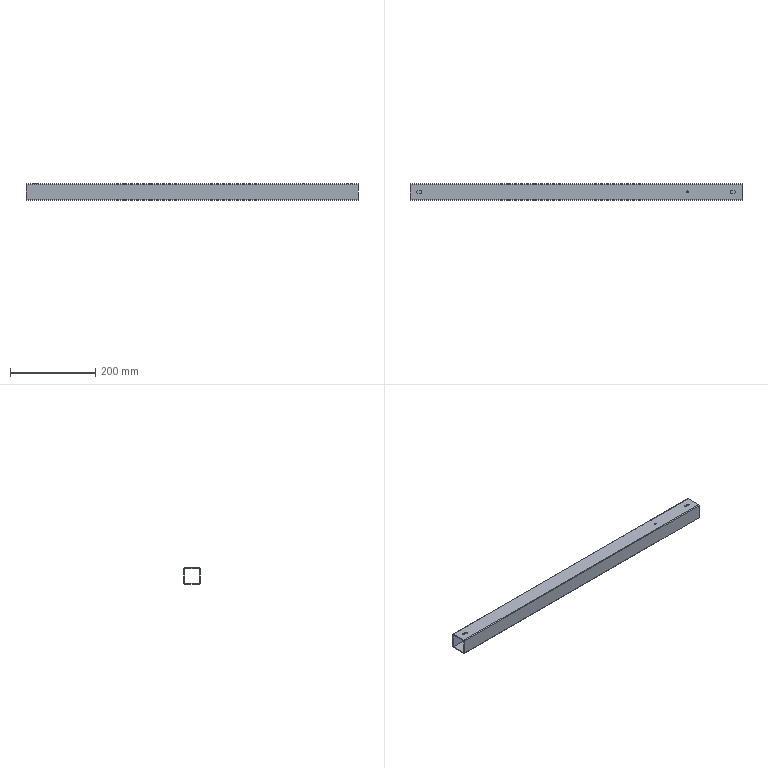Part | NX | features BREP 1 | 1 solid | 26 faces | box 780.034 x 38.1 x 38.1 mm | volume 210452 mm3 | plane 14 | cylinder 12 | commonest cylinder face diameters 5.715 x6 3.175 x4 4.699 x2
STEP:
#1=CARTESIAN_POINT('',(-390.017,19.05,-17.462));
#2=VERTEX_POINT('',#1);
#3=CARTESIAN_POINT('',(-390.017,19.05,17.462));
#4=VERTEX_POINT('',#3);
#5=CARTESIAN_POINT('',(-390.017,19.05,-17.462));
#6=DIRECTION('',(0.,0.,1.));
#7=VECTOR('',#6,1000.);
#8=LINE('',#5,#7);
#9=EDGE_CURVE('',#2,#4,#8,.T.);
#10=ORIENTED_EDGE('',*,*,#9,.F.);
#11=CARTESIAN_POINT('',(-390.017,17.462,-19.05));
#12=VERTEX_POINT('',#11);
#13=CARTESIAN_POINT('',(-390.017,17.462,-17.462));
#14=DIRECTION('',(-1.,0.,0.));
#15=DIRECTION('',(0.,1.,0.));
#16=AXIS2_PLACEMENT_3D('',#13,#14,#15);
#17=CIRCLE('',#16,1.587);
#18=EDGE_CURVE('',#2,#12,#17,.T.);
#19=ORIENTED_EDGE('',*,*,#18,.T.);
#20=CARTESIAN_POINT('',(-390.017,-17.462,-19.05));
#21=VERTEX_POINT('',#20);
#22=CARTESIAN_POINT('',(-390.017,-17.462,-19.05));
#23=DIRECTION('',(0.,1.,0.));
#24=VECTOR('',#23,1000.);
#25=LINE('',#22,#24);
#26=EDGE_CURVE('',#21,#12,#25,.T.);
#27=ORIENTED_EDGE('',*,*,#26,.F.);
#28=CARTESIAN_POINT('',(-390.017,-19.05,-17.462));
#29=VERTEX_POINT('',#28);
#30=CARTESIAN_POINT('',(-390.017,-17.462,-17.462));
#31=DIRECTION('',(-1.,0.,0.));
#32=DIRECTION('',(0.,0.,-1.));
#33=AXIS2_PLACEMENT_3D('',#30,#31,#32);
#34=CIRCLE('',#33,1.587);
#35=EDGE_CURVE('',#21,#29,#34,.T.);
#36=ORIENTED_EDGE('',*,*,#35,.T.);
#37=CARTESIAN_POINT('',(-390.017,-19.05,17.462));
#38=VERTEX_POINT('',#37);
#39=CARTESIAN_POINT('',(-390.017,-19.05,17.462));
#40=DIRECTION('',(0.,0.,-1.));
#41=VECTOR('',#40,1000.);
#42=LINE('',#39,#41);
#43=EDGE_CURVE('',#38,#29,#42,.T.);
#44=ORIENTED_EDGE('',*,*,#43,.F.);
#45=CARTESIAN_POINT('',(-390.017,-17.462,19.05));
#46=VERTEX_POINT('',#45);
#47=CARTESIAN_POINT('',(-390.017,-17.462,17.462));
#48=DIRECTION('',(-1.,0.,0.));
#49=DIRECTION('',(0.,-1.,0.));
#50=AXIS2_PLACEMENT_3D('',#47,#48,#49);
#51=CIRCLE('',#50,1.587);
#52=EDGE_CURVE('',#38,#46,#51,.T.);
#53=ORIENTED_EDGE('',*,*,#52,.T.);
#54=CARTESIAN_POINT('',(-390.017,17.462,19.05));
#55=VERTEX_POINT('',#54);
#56=CARTESIAN_POINT('',(-390.017,17.462,19.05));
#57=DIRECTION('',(0.,-1.,0.));
#58=VECTOR('',#57,1000.);
#59=LINE('',#56,#58);
#60=EDGE_CURVE('',#55,#46,#59,.T.);
#61=ORIENTED_EDGE('',*,*,#60,.F.);
#62=CARTESIAN_POINT('',(-390.017,17.462,17.462));
#63=DIRECTION('',(-1.,0.,0.));
#64=DIRECTION('',(0.,0.,1.));
#65=AXIS2_PLACEMENT_3D('',#62,#63,#64);
#66=CIRCLE('',#65,1.587);
#67=EDGE_CURVE('',#55,#4,#66,.T.);
#68=ORIENTED_EDGE('',*,*,#67,.T.);
#69=EDGE_LOOP('',(#10,#19,#27,#36,#44,#53,#61,#68));
#70=FACE_BOUND('',#69,.T.);
#71=CARTESIAN_POINT('',(-390.017,17.17,17.17));
#72=VERTEX_POINT('',#71);
#73=CARTESIAN_POINT('',(-390.017,17.17,-17.17));
#74=VERTEX_POINT('',#73);
#75=CARTESIAN_POINT('',(-390.017,17.17,17.17));
#76=DIRECTION('',(0.,0.,-1.));
#77=VECTOR('',#76,1000.);
#78=LINE('',#75,#77);
#79=EDGE_CURVE('',#72,#74,#78,.T.);
#80=ORIENTED_EDGE('',*,*,#79,.F.);
#81=CARTESIAN_POINT('',(-390.017,-17.17,17.17));
#82=VERTEX_POINT('',#81);
#83=CARTESIAN_POINT('',(-390.017,-17.17,17.17));
#84=DIRECTION('',(0.,1.,0.));
#85=VECTOR('',#84,1000.);
#86=LINE('',#83,#85);
#87=EDGE_CURVE('',#82,#72,#86,.T.);
#88=ORIENTED_EDGE('',*,*,#87,.F.);
#89=CARTESIAN_POINT('',(-390.017,-17.17,-17.17));
#90=VERTEX_POINT('',#89);
#91=CARTESIAN_POINT('',(-390.017,-17.17,-17.17));
#92=DIRECTION('',(0.,0.,1.));
#93=VECTOR('',#92,1000.);
#94=LINE('',#91,#93);
#95=EDGE_CURVE('',#90,#82,#94,.T.);
#96=ORIENTED_EDGE('',*,*,#95,.F.);
#97=CARTESIAN_POINT('',(-390.017,17.17,-17.17));
#98=DIRECTION('',(0.,-1.,0.));
#99=VECTOR('',#98,1000.);
#100=LINE('',#97,#99);
#101=EDGE_CURVE('',#74,#90,#100,.T.);
#102=ORIENTED_EDGE('',*,*,#101,.F.);
#103=EDGE_LOOP('',(#80,#88,#96,#102));
#104=FACE_BOUND('',#103,.T.);
#105=CARTESIAN_POINT('',(-390.017,0.,0.));
#106=DIRECTION('',(1.,0.,0.));
#107=DIRECTION('',(0.,1.,0.));
#108=AXIS2_PLACEMENT_3D('',#105,#106,#107);
#109=PLANE('',#108);
#110=ADVANCED_FACE('',(#70,#104),#109,.F.);
#111=CARTESIAN_POINT('',(390.017,-17.17,-17.17));
#112=VERTEX_POINT('',#111);
#113=CARTESIAN_POINT('',(-390.017,-17.17,-17.17));
#114=DIRECTION('',(1.,0.,0.));
#115=VECTOR('',#114,1000.);
#116=LINE('',#113,#115);
#117=EDGE_CURVE('',#90,#112,#116,.T.);
#118=ORIENTED_EDGE('',*,*,#117,.T.);
#119=CARTESIAN_POINT('',(390.017,17.17,-17.17));
#120=VERTEX_POINT('',#119);
#121=CARTESIAN_POINT('',(390.017,17.17,-17.17));
#122=DIRECTION('',(0.,-1.,0.));
#123=VECTOR('',#122,1000.);
#124=LINE('',#121,#123);
#125=EDGE_CURVE('',#120,#112,#124,.T.);
#126=ORIENTED_EDGE('',*,*,#125,.F.);
#127=CARTESIAN_POINT('',(-390.017,17.17,-17.17));
#128=DIRECTION('',(1.,0.,0.));
#129=VECTOR('',#128,1000.);
#130=LINE('',#127,#129);
#131=EDGE_CURVE('',#74,#120,#130,.T.);
#132=ORIENTED_EDGE('',*,*,#131,.F.);
#133=ORIENTED_EDGE('',*,*,#101,.T.);
#134=EDGE_LOOP('',(#118,#126,#132,#133));
#135=FACE_BOUND('',#134,.T.);
#136=CARTESIAN_POINT('',(-390.017,17.17,-17.17));
#137=DIRECTION('',(0.,0.,1.));
#138=DIRECTION('',(1.,0.,0.));
#139=AXIS2_PLACEMENT_3D('',#136,#137,#138);
#140=PLANE('',#139);
#141=ADVANCED_FACE('',(#135),#140,.T.);
#142=ORIENTED_EDGE('',*,*,#131,.T.);
#143=CARTESIAN_POINT('',(390.017,17.17,17.17));
#144=VERTEX_POINT('',#143);
#145=CARTESIAN_POINT('',(390.017,17.17,17.17));
#146=DIRECTION('',(0.,0.,-1.));
#147=VECTOR('',#146,1000.);
#148=LINE('',#145,#147);
#149=EDGE_CURVE('',#144,#120,#148,.T.);
#150=ORIENTED_EDGE('',*,*,#149,.F.);
#151=CARTESIAN_POINT('',(-390.017,17.17,17.17));
#152=DIRECTION('',(1.,0.,0.));
#153=VECTOR('',#152,1000.);
#154=LINE('',#151,#153);
#155=EDGE_CURVE('',#72,#144,#154,.T.);
#156=ORIENTED_EDGE('',*,*,#155,.F.);
#157=ORIENTED_EDGE('',*,*,#79,.T.);
#158=EDGE_LOOP('',(#142,#150,#156,#157));
#159=FACE_BOUND('',#158,.T.);
#160=CARTESIAN_POINT('',(-390.017,17.17,17.17));
#161=DIRECTION('',(0.,-1.,0.));
#162=DIRECTION('',(0.,0.,-1.));
#163=AXIS2_PLACEMENT_3D('',#160,#161,#162);
#164=PLANE('',#163);
#165=ADVANCED_FACE('',(#159),#164,.T.);
#166=ORIENTED_EDGE('',*,*,#155,.T.);
#167=CARTESIAN_POINT('',(390.017,-17.17,17.17));
#168=VERTEX_POINT('',#167);
#169=CARTESIAN_POINT('',(390.017,-17.17,17.17));
#170=DIRECTION('',(0.,1.,0.));
#171=VECTOR('',#170,1000.);
#172=LINE('',#169,#171);
#173=EDGE_CURVE('',#168,#144,#172,.T.);
#174=ORIENTED_EDGE('',*,*,#173,.F.);
#175=CARTESIAN_POINT('',(-390.017,-17.17,17.17));
#176=DIRECTION('',(1.,0.,0.));
#177=VECTOR('',#176,1000.);
#178=LINE('',#175,#177);
#179=EDGE_CURVE('',#82,#168,#178,.T.);
#180=ORIENTED_EDGE('',*,*,#179,.F.);
#181=ORIENTED_EDGE('',*,*,#87,.T.);
#182=EDGE_LOOP('',(#166,#174,#180,#181));
#183=FACE_BOUND('',#182,.T.);
#184=CARTESIAN_POINT('',(364.935,-2.857,17.17));
#185=VERTEX_POINT('',#184);
#186=CARTESIAN_POINT('',(371.92,-2.857,17.17));
#187=VERTEX_POINT('',#186);
#188=CARTESIAN_POINT('',(364.935,-2.857,17.17));
#189=DIRECTION('',(1.,0.,0.));
#190=VECTOR('',#189,1000.);
#191=LINE('',#188,#190);
#192=EDGE_CURVE('',#185,#187,#191,.T.);
#193=ORIENTED_EDGE('',*,*,#192,.T.);
#194=CARTESIAN_POINT('',(374.777,0.,17.17));
#195=VERTEX_POINT('',#194);
#196=CARTESIAN_POINT('',(371.92,0.,17.17));
#197=DIRECTION('',(0.,0.,1.));
#198=DIRECTION('',(0.,-1.,0.));
#199=AXIS2_PLACEMENT_3D('',#196,#197,#198);
#200=CIRCLE('',#199,2.857);
#201=EDGE_CURVE('',#187,#195,#200,.T.);
#202=ORIENTED_EDGE('',*,*,#201,.T.);
#203=CARTESIAN_POINT('',(371.92,2.857,17.17));
#204=VERTEX_POINT('',#203);
#205=CARTESIAN_POINT('',(371.92,0.,17.17));
#206=DIRECTION('',(0.,0.,1.));
#207=DIRECTION('',(0.,-1.,0.));
#208=AXIS2_PLACEMENT_3D('',#205,#206,#207);
#209=CIRCLE('',#208,2.857);
#210=EDGE_CURVE('',#195,#204,#209,.T.);
#211=ORIENTED_EDGE('',*,*,#210,.T.);
#212=CARTESIAN_POINT('',(364.935,2.857,17.17));
#213=VERTEX_POINT('',#212);
#214=CARTESIAN_POINT('',(371.92,2.857,17.17));
#215=DIRECTION('',(-1.,0.,0.));
#216=VECTOR('',#215,1000.);
#217=LINE('',#214,#216);
#218=EDGE_CURVE('',#204,#213,#217,.T.);
#219=ORIENTED_EDGE('',*,*,#218,.T.);
#220=CARTESIAN_POINT('',(364.935,0.,17.17));
#221=DIRECTION('',(0.,0.,1.));
#222=DIRECTION('',(0.,1.,0.));
#223=AXIS2_PLACEMENT_3D('',#220,#221,#222);
#224=CIRCLE('',#223,2.857);
#225=EDGE_CURVE('',#213,#185,#224,.T.);
#226=ORIENTED_EDGE('',*,*,#225,.T.);
#227=EDGE_LOOP('',(#193,#202,#211,#219,#226));
#228=FACE_BOUND('',#227,.T.);
#229=CARTESIAN_POINT('',(-371.92,2.857,17.17));
#230=VERTEX_POINT('',#229);
#231=CARTESIAN_POINT('',(-364.935,2.857,17.17));
#232=VERTEX_POINT('',#231);
#233=CARTESIAN_POINT('',(-371.92,2.857,17.17));
#234=DIRECTION('',(1.,0.,0.));
#235=VECTOR('',#234,1000.);
#236=LINE('',#233,#235);
#237=EDGE_CURVE('',#230,#232,#236,.T.);
#238=ORIENTED_EDGE('',*,*,#237,.F.);
#239=CARTESIAN_POINT('',(-374.777,0.,17.17));
#240=VERTEX_POINT('',#239);
#241=CARTESIAN_POINT('',(-371.92,0.,17.17));
#242=DIRECTION('',(0.,0.,-1.));
#243=DIRECTION('',(0.,-1.,0.));
#244=AXIS2_PLACEMENT_3D('',#241,#242,#243);
#245=CIRCLE('',#244,2.857);
#246=EDGE_CURVE('',#240,#230,#245,.T.);
#247=ORIENTED_EDGE('',*,*,#246,.F.);
#248=CARTESIAN_POINT('',(-371.92,-2.857,17.17));
#249=VERTEX_POINT('',#248);
#250=CARTESIAN_POINT('',(-371.92,0.,17.17));
#251=DIRECTION('',(0.,0.,-1.));
#252=DIRECTION('',(0.,-1.,0.));
#253=AXIS2_PLACEMENT_3D('',#250,#251,#252);
#254=CIRCLE('',#253,2.857);
#255=EDGE_CURVE('',#249,#240,#254,.T.);
#256=ORIENTED_EDGE('',*,*,#255,.F.);
#257=CARTESIAN_POINT('',(-364.935,-2.857,17.17));
#258=VERTEX_POINT('',#257);
#259=CARTESIAN_POINT('',(-364.935,-2.857,17.17));
#260=DIRECTION('',(-1.,0.,0.));
#261=VECTOR('',#260,1000.);
#262=LINE('',#259,#261);
#263=EDGE_CURVE('',#258,#249,#262,.T.);
#264=ORIENTED_EDGE('',*,*,#263,.F.);
#265=CARTESIAN_POINT('',(-364.935,0.,17.17));
#266=DIRECTION('',(0.,0.,-1.));
#267=DIRECTION('',(0.,1.,0.));
#268=AXIS2_PLACEMENT_3D('',#265,#266,#267);
#269=CIRCLE('',#268,2.857);
#270=EDGE_CURVE('',#232,#258,#269,.T.);
#271=ORIENTED_EDGE('',*,*,#270,.F.);
#272=EDGE_LOOP('',(#238,#247,#256,#264,#271));
#273=FACE_BOUND('',#272,.T.);
#274=CARTESIAN_POINT('',(263.017,2.349,17.17));
#275=VERTEX_POINT('',#274);
#276=CARTESIAN_POINT('',(263.017,-2.349,17.17));
#277=VERTEX_POINT('',#276);
#278=CARTESIAN_POINT('',(263.017,0.,17.17));
#279=DIRECTION('',(0.,0.,1.));
#280=DIRECTION('',(0.,1.,0.));
#281=AXIS2_PLACEMENT_3D('',#278,#279,#280);
#282=CIRCLE('',#281,2.349);
#283=EDGE_CURVE('',#275,#277,#282,.T.);
#284=ORIENTED_EDGE('',*,*,#283,.T.);
#285=CARTESIAN_POINT('',(263.017,0.,17.17));
#286=DIRECTION('',(0.,0.,1.));
#287=DIRECTION('',(0.,-1.,0.));
#288=AXIS2_PLACEMENT_3D('',#285,#286,#287);
#289=CIRCLE('',#288,2.349);
#290=EDGE_CURVE('',#277,#275,#289,.T.);
#291=ORIENTED_EDGE('',*,*,#290,.T.);
#292=EDGE_LOOP('',(#284,#291));
#293=FACE_BOUND('',#292,.T.);
#294=CARTESIAN_POINT('',(-390.017,-17.17,17.17));
#295=DIRECTION('',(0.,0.,-1.));
#296=DIRECTION('',(0.,-1.,0.));
#297=AXIS2_PLACEMENT_3D('',#294,#295,#296);
#298=PLANE('',#297);
#299=ADVANCED_FACE('',(#183,#228,#273,#293),#298,.T.);
#300=ORIENTED_EDGE('',*,*,#179,.T.);
#301=CARTESIAN_POINT('',(390.017,-17.17,-17.17));
#302=DIRECTION('',(0.,0.,1.));
#303=VECTOR('',#302,1000.);
#304=LINE('',#301,#303);
#305=EDGE_CURVE('',#112,#168,#304,.T.);
#306=ORIENTED_EDGE('',*,*,#305,.F.);
#307=ORIENTED_EDGE('',*,*,#117,.F.);
#308=ORIENTED_EDGE('',*,*,#95,.T.);
#309=EDGE_LOOP('',(#300,#306,#307,#308));
#310=FACE_BOUND('',#309,.T.);
#311=CARTESIAN_POINT('',(-390.017,-17.17,-17.17));
#312=DIRECTION('',(0.,1.,0.));
#313=DIRECTION('',(1.,0.,0.));
#314=AXIS2_PLACEMENT_3D('',#311,#312,#313);
#315=PLANE('',#314);
#316=ADVANCED_FACE('',(#310),#315,.T.);
#317=CARTESIAN_POINT('',(390.017,17.462,19.05));
#318=VERTEX_POINT('',#317);
#319=CARTESIAN_POINT('',(390.017,-17.462,19.05));
#320=VERTEX_POINT('',#319);
#321=CARTESIAN_POINT('',(390.017,17.462,19.05));
#322=DIRECTION('',(0.,-1.,0.));
#323=VECTOR('',#322,1000.);
#324=LINE('',#321,#323);
#325=EDGE_CURVE('',#318,#320,#324,.T.);
#326=ORIENTED_EDGE('',*,*,#325,.T.);
#327=CARTESIAN_POINT('',(390.017,-19.05,17.462));
#328=VERTEX_POINT('',#327);
#329=CARTESIAN_POINT('',(390.017,-17.462,17.462));
#330=DIRECTION('',(1.,0.,0.));
#331=DIRECTION('',(0.,0.,1.));
#332=AXIS2_PLACEMENT_3D('',#329,#330,#331);
#333=CIRCLE('',#332,1.587);
#334=EDGE_CURVE('',#320,#328,#333,.T.);
#335=ORIENTED_EDGE('',*,*,#334,.T.);
#336=CARTESIAN_POINT('',(390.017,-19.05,-17.462));
#337=VERTEX_POINT('',#336);
#338=CARTESIAN_POINT('',(390.017,-19.05,17.462));
#339=DIRECTION('',(0.,0.,-1.));
#340=VECTOR('',#339,1000.);
#341=LINE('',#338,#340);
#342=EDGE_CURVE('',#328,#337,#341,.T.);
#343=ORIENTED_EDGE('',*,*,#342,.T.);
#344=CARTESIAN_POINT('',(390.017,-17.462,-19.05));
#345=VERTEX_POINT('',#344);
#346=CARTESIAN_POINT('',(390.017,-17.462,-17.462));
#347=DIRECTION('',(1.,0.,0.));
#348=DIRECTION('',(0.,-1.,0.));
#349=AXIS2_PLACEMENT_3D('',#346,#347,#348);
#350=CIRCLE('',#349,1.587);
#351=EDGE_CURVE('',#337,#345,#350,.T.);
#352=ORIENTED_EDGE('',*,*,#351,.T.);
#353=CARTESIAN_POINT('',(390.017,17.462,-19.05));
#354=VERTEX_POINT('',#353);
#355=CARTESIAN_POINT('',(390.017,-17.462,-19.05));
#356=DIRECTION('',(0.,1.,0.));
#357=VECTOR('',#356,1000.);
#358=LINE('',#355,#357);
#359=EDGE_CURVE('',#345,#354,#358,.T.);
#360=ORIENTED_EDGE('',*,*,#359,.T.);
#361=CARTESIAN_POINT('',(390.017,19.05,-17.462));
#362=VERTEX_POINT('',#361);
#363=CARTESIAN_POINT('',(390.017,17.462,-17.462));
#364=DIRECTION('',(1.,0.,0.));
#365=DIRECTION('',(0.,0.,-1.));
#366=AXIS2_PLACEMENT_3D('',#363,#364,#365);
#367=CIRCLE('',#366,1.587);
#368=EDGE_CURVE('',#354,#362,#367,.T.);
#369=ORIENTED_EDGE('',*,*,#368,.T.);
#370=CARTESIAN_POINT('',(390.017,19.05,17.462));
#371=VERTEX_POINT('',#370);
#372=CARTESIAN_POINT('',(390.017,19.05,-17.462));
#373=DIRECTION('',(0.,0.,1.));
#374=VECTOR('',#373,1000.);
#375=LINE('',#372,#374);
#376=EDGE_CURVE('',#362,#371,#375,.T.);
#377=ORIENTED_EDGE('',*,*,#376,.T.);
#378=CARTESIAN_POINT('',(390.017,17.462,17.462));
#379=DIRECTION('',(1.,0.,0.));
#380=DIRECTION('',(0.,1.,0.));
#381=AXIS2_PLACEMENT_3D('',#378,#379,#380);
#382=CIRCLE('',#381,1.587);
#383=EDGE_CURVE('',#371,#318,#382,.T.);
#384=ORIENTED_EDGE('',*,*,#383,.T.);
#385=EDGE_LOOP('',(#326,#335,#343,#352,#360,#369,#377,#384));
#386=FACE_BOUND('',#385,.T.);
#387=ORIENTED_EDGE('',*,*,#305,.T.);
#388=ORIENTED_EDGE('',*,*,#173,.T.);
#389=ORIENTED_EDGE('',*,*,#149,.T.);
#390=ORIENTED_EDGE('',*,*,#125,.T.);
#391=EDGE_LOOP('',(#387,#388,#389,#390));
#392=FACE_BOUND('',#391,.T.);
#393=CARTESIAN_POINT('',(390.017,0.,0.));
#394=DIRECTION('',(1.,0.,0.));
#395=DIRECTION('',(0.,1.,0.));
#396=AXIS2_PLACEMENT_3D('',#393,#394,#395);
#397=PLANE('',#396);
#398=ADVANCED_FACE('',(#386,#392),#397,.T.);
#399=ORIENTED_EDGE('',*,*,#383,.F.);
#400=CARTESIAN_POINT('',(390.017,19.05,17.462));
#401=DIRECTION('',(-1.,0.,0.));
#402=VECTOR('',#401,1000.);
#403=LINE('',#400,#402);
#404=EDGE_CURVE('',#371,#4,#403,.T.);
#405=ORIENTED_EDGE('',*,*,#404,.T.);
#406=ORIENTED_EDGE('',*,*,#67,.F.);
#407=CARTESIAN_POINT('',(390.017,17.462,19.05));
#408=DIRECTION('',(-1.,0.,0.));
#409=VECTOR('',#408,1000.);
#410=LINE('',#407,#409);
#411=EDGE_CURVE('',#318,#55,#410,.T.);
#412=ORIENTED_EDGE('',*,*,#411,.F.);
#413=EDGE_LOOP('',(#399,#405,#406,#412));
#414=FACE_BOUND('',#413,.T.);
#415=CARTESIAN_POINT('',(391.24,17.462,17.462));
#416=DIRECTION('',(-1.,0.,0.));
#417=DIRECTION('',(0.,0.,1.));
#418=AXIS2_PLACEMENT_3D('',#415,#416,#417);
#419=CYLINDRICAL_SURFACE('',#418,1.587);
#420=ADVANCED_FACE('',(#414),#419,.T.);
#421=ORIENTED_EDGE('',*,*,#60,.T.);
#422=CARTESIAN_POINT('',(390.017,-17.462,19.05));
#423=DIRECTION('',(-1.,0.,0.));
#424=VECTOR('',#423,1000.);
#425=LINE('',#422,#424);
#426=EDGE_CURVE('',#320,#46,#425,.T.);
#427=ORIENTED_EDGE('',*,*,#426,.F.);
#428=ORIENTED_EDGE('',*,*,#325,.F.);
#429=ORIENTED_EDGE('',*,*,#411,.T.);
#430=EDGE_LOOP('',(#421,#427,#428,#429));
#431=FACE_BOUND('',#430,.T.);
#432=CARTESIAN_POINT('',(371.92,2.857,19.05));
#433=VERTEX_POINT('',#432);
#434=CARTESIAN_POINT('',(364.935,2.857,19.05));
#435=VERTEX_POINT('',#434);
#436=CARTESIAN_POINT('',(371.92,2.857,19.05));
#437=DIRECTION('',(-1.,0.,0.));
#438=VECTOR('',#437,1000.);
#439=LINE('',#436,#438);
#440=EDGE_CURVE('',#433,#435,#439,.T.);
#441=ORIENTED_EDGE('',*,*,#440,.F.);
#442=CARTESIAN_POINT('',(374.777,0.,19.05));
#443=VERTEX_POINT('',#442);
#444=CARTESIAN_POINT('',(371.92,0.,19.05));
#445=DIRECTION('',(0.,0.,1.));
#446=DIRECTION('',(0.,-1.,0.));
#447=AXIS2_PLACEMENT_3D('',#444,#445,#446);
#448=CIRCLE('',#447,2.857);
#449=EDGE_CURVE('',#443,#433,#448,.T.);
#450=ORIENTED_EDGE('',*,*,#449,.F.);
#451=CARTESIAN_POINT('',(371.92,-2.857,19.05));
#452=VERTEX_POINT('',#451);
#453=CARTESIAN_POINT('',(371.92,0.,19.05));
#454=DIRECTION('',(0.,0.,1.));
#455=DIRECTION('',(0.,-1.,0.));
#456=AXIS2_PLACEMENT_3D('',#453,#454,#455);
#457=CIRCLE('',#456,2.857);
#458=EDGE_CURVE('',#452,#443,#457,.T.);
#459=ORIENTED_EDGE('',*,*,#458,.F.);
#460=CARTESIAN_POINT('',(364.935,-2.857,19.05));
#461=VERTEX_POINT('',#460);
#462=CARTESIAN_POINT('',(364.935,-2.857,19.05));
#463=DIRECTION('',(1.,0.,0.));
#464=VECTOR('',#463,1000.);
#465=LINE('',#462,#464);
#466=EDGE_CURVE('',#461,#452,#465,.T.);
#467=ORIENTED_EDGE('',*,*,#466,.F.);
#468=CARTESIAN_POINT('',(364.935,0.,19.05));
#469=DIRECTION('',(0.,0.,1.));
#470=DIRECTION('',(0.,1.,0.));
#471=AXIS2_PLACEMENT_3D('',#468,#469,#470);
#472=CIRCLE('',#471,2.857);
#473=EDGE_CURVE('',#435,#461,#472,.T.);
#474=ORIENTED_EDGE('',*,*,#473,.F.);
#475=EDGE_LOOP('',(#441,#450,#459,#467,#474));
#476=FACE_BOUND('',#475,.T.);
#477=CARTESIAN_POINT('',(-364.935,-2.857,19.05));
#478=VERTEX_POINT('',#477);
#479=CARTESIAN_POINT('',(-371.92,-2.857,19.05));
#480=VERTEX_POINT('',#479);
#481=CARTESIAN_POINT('',(-364.935,-2.857,19.05));
#482=DIRECTION('',(-1.,0.,0.));
#483=VECTOR('',#482,1000.);
#484=LINE('',#481,#483);
#485=EDGE_CURVE('',#478,#480,#484,.T.);
#486=ORIENTED_EDGE('',*,*,#485,.T.);
#487=CARTESIAN_POINT('',(-374.777,0.,19.05));
#488=VERTEX_POINT('',#487);
#489=CARTESIAN_POINT('',(-371.92,0.,19.05));
#490=DIRECTION('',(0.,0.,-1.));
#491=DIRECTION('',(0.,-1.,0.));
#492=AXIS2_PLACEMENT_3D('',#489,#490,#491);
#493=CIRCLE('',#492,2.857);
#494=EDGE_CURVE('',#480,#488,#493,.T.);
#495=ORIENTED_EDGE('',*,*,#494,.T.);
#496=CARTESIAN_POINT('',(-371.92,2.857,19.05));
#497=VERTEX_POINT('',#496);
#498=CARTESIAN_POINT('',(-371.92,0.,19.05));
#499=DIRECTION('',(0.,0.,-1.));
#500=DIRECTION('',(0.,-1.,0.));
#501=AXIS2_PLACEMENT_3D('',#498,#499,#500);
#502=CIRCLE('',#501,2.857);
#503=EDGE_CURVE('',#488,#497,#502,.T.);
#504=ORIENTED_EDGE('',*,*,#503,.T.);
#505=CARTESIAN_POINT('',(-364.935,2.857,19.05));
#506=VERTEX_POINT('',#505);
#507=CARTESIAN_POINT('',(-371.92,2.857,19.05));
#508=DIRECTION('',(1.,0.,0.));
#509=VECTOR('',#508,1000.);
#510=LINE('',#507,#509);
#511=EDGE_CURVE('',#497,#506,#510,.T.);
#512=ORIENTED_EDGE('',*,*,#511,.T.);
#513=CARTESIAN_POINT('',(-364.935,0.,19.05));
#514=DIRECTION('',(0.,0.,-1.));
#515=DIRECTION('',(0.,1.,0.));
#516=AXIS2_PLACEMENT_3D('',#513,#514,#515);
#517=CIRCLE('',#516,2.857);
#518=EDGE_CURVE('',#506,#478,#517,.T.);
#519=ORIENTED_EDGE('',*,*,#518,.T.);
#520=EDGE_LOOP('',(#486,#495,#504,#512,#519));
#521=FACE_BOUND('',#520,.T.);
#522=CARTESIAN_POINT('',(263.017,2.349,19.05));
#523=VERTEX_POINT('',#522);
#524=CARTESIAN_POINT('',(263.017,-2.349,19.05));
#525=VERTEX_POINT('',#524);
#526=CARTESIAN_POINT('',(263.017,0.,19.05));
#527=DIRECTION('',(0.,0.,1.));
#528=DIRECTION('',(0.,1.,0.));
#529=AXIS2_PLACEMENT_3D('',#526,#527,#528);
#530=CIRCLE('',#529,2.349);
#531=EDGE_CURVE('',#523,#525,#530,.T.);
#532=ORIENTED_EDGE('',*,*,#531,.F.);
#533=CARTESIAN_POINT('',(263.017,0.,19.05));
#534=DIRECTION('',(0.,0.,1.));
#535=DIRECTION('',(0.,-1.,0.));
#536=AXIS2_PLACEMENT_3D('',#533,#534,#535);
#537=CIRCLE('',#536,2.349);
#538=EDGE_CURVE('',#525,#523,#537,.T.);
#539=ORIENTED_EDGE('',*,*,#538,.F.);
#540=EDGE_LOOP('',(#532,#539));
#541=FACE_BOUND('',#540,.T.);
#542=CARTESIAN_POINT('',(-390.017,19.05,19.05));
#543=DIRECTION('',(0.,0.,1.));
#544=DIRECTION('',(1.,0.,0.));
#545=AXIS2_PLACEMENT_3D('',#542,#543,#544);
#546=PLANE('',#545);
#547=ADVANCED_FACE('',(#431,#476,#521,#541),#546,.T.);
#548=ORIENTED_EDGE('',*,*,#334,.F.);
#549=ORIENTED_EDGE('',*,*,#426,.T.);
#550=ORIENTED_EDGE('',*,*,#52,.F.);
#551=CARTESIAN_POINT('',(390.017,-19.05,17.462));
#552=DIRECTION('',(-1.,0.,0.));
#553=VECTOR('',#552,1000.);
#554=LINE('',#551,#553);
#555=EDGE_CURVE('',#328,#38,#554,.T.);
#556=ORIENTED_EDGE('',*,*,#555,.F.);
#557=EDGE_LOOP('',(#548,#549,#550,#556));
#558=FACE_BOUND('',#557,.T.);
#559=CARTESIAN_POINT('',(391.24,-17.462,17.462));
#560=DIRECTION('',(-1.,0.,0.));
#561=DIRECTION('',(0.,-1.,0.));
#562=AXIS2_PLACEMENT_3D('',#559,#560,#561);
#563=CYLINDRICAL_SURFACE('',#562,1.587);
#564=ADVANCED_FACE('',(#558),#563,.T.);
#565=ORIENTED_EDGE('',*,*,#43,.T.);
#566=CARTESIAN_POINT('',(390.017,-19.05,-17.462));
#567=DIRECTION('',(-1.,0.,0.));
#568=VECTOR('',#567,1000.);
#569=LINE('',#566,#568);
#570=EDGE_CURVE('',#337,#29,#569,.T.);
#571=ORIENTED_EDGE('',*,*,#570,.F.);
#572=ORIENTED_EDGE('',*,*,#342,.F.);
#573=ORIENTED_EDGE('',*,*,#555,.T.);
#574=EDGE_LOOP('',(#565,#571,#572,#573));
#575=FACE_BOUND('',#574,.T.);
#576=CARTESIAN_POINT('',(-390.017,-19.05,19.05));
#577=DIRECTION('',(0.,-1.,0.));
#578=DIRECTION('',(0.,0.,-1.));
#579=AXIS2_PLACEMENT_3D('',#576,#577,#578);
#580=PLANE('',#579);
#581=ADVANCED_FACE('',(#575),#580,.T.);
#582=ORIENTED_EDGE('',*,*,#351,.F.);
#583=ORIENTED_EDGE('',*,*,#570,.T.);
#584=ORIENTED_EDGE('',*,*,#35,.F.);
#585=CARTESIAN_POINT('',(390.017,-17.462,-19.05));
#586=DIRECTION('',(-1.,0.,0.));
#587=VECTOR('',#586,1000.);
#588=LINE('',#585,#587);
#589=EDGE_CURVE('',#345,#21,#588,.T.);
#590=ORIENTED_EDGE('',*,*,#589,.F.);
#591=EDGE_LOOP('',(#582,#583,#584,#590));
#592=FACE_BOUND('',#591,.T.);
#593=CARTESIAN_POINT('',(391.24,-17.462,-17.462));
#594=DIRECTION('',(-1.,0.,0.));
#595=DIRECTION('',(0.,0.,-1.));
#596=AXIS2_PLACEMENT_3D('',#593,#594,#595);
#597=CYLINDRICAL_SURFACE('',#596,1.587);
#598=ADVANCED_FACE('',(#592),#597,.T.);
#599=ORIENTED_EDGE('',*,*,#359,.F.);
#600=ORIENTED_EDGE('',*,*,#589,.T.);
#601=ORIENTED_EDGE('',*,*,#26,.T.);
#602=CARTESIAN_POINT('',(390.017,17.462,-19.05));
#603=DIRECTION('',(-1.,0.,0.));
#604=VECTOR('',#603,1000.);
#605=LINE('',#602,#604);
#606=EDGE_CURVE('',#354,#12,#605,.T.);
#607=ORIENTED_EDGE('',*,*,#606,.F.);
#608=EDGE_LOOP('',(#599,#600,#601,#607));
#609=FACE_BOUND('',#608,.T.);
#610=CARTESIAN_POINT('',(-390.017,-19.05,-19.05));
#611=DIRECTION('',(0.,0.,-1.));
#612=DIRECTION('',(0.,-1.,0.));
#613=AXIS2_PLACEMENT_3D('',#610,#611,#612);
#614=PLANE('',#613);
#615=ADVANCED_FACE('',(#609),#614,.T.);
#616=ORIENTED_EDGE('',*,*,#368,.F.);
#617=ORIENTED_EDGE('',*,*,#606,.T.);
#618=ORIENTED_EDGE('',*,*,#18,.F.);
#619=CARTESIAN_POINT('',(390.017,19.05,-17.462));
#620=DIRECTION('',(-1.,0.,0.));
#621=VECTOR('',#620,1000.);
#622=LINE('',#619,#621);
#623=EDGE_CURVE('',#362,#2,#622,.T.);
#624=ORIENTED_EDGE('',*,*,#623,.F.);
#625=EDGE_LOOP('',(#616,#617,#618,#624));
#626=FACE_BOUND('',#625,.T.);
#627=CARTESIAN_POINT('',(391.24,17.462,-17.462));
#628=DIRECTION('',(-1.,0.,0.));
#629=DIRECTION('',(0.,1.,0.));
#630=AXIS2_PLACEMENT_3D('',#627,#628,#629);
#631=CYLINDRICAL_SURFACE('',#630,1.587);
#632=ADVANCED_FACE('',(#626),#631,.T.);
#633=ORIENTED_EDGE('',*,*,#376,.F.);
#634=ORIENTED_EDGE('',*,*,#623,.T.);
#635=ORIENTED_EDGE('',*,*,#9,.T.);
#636=ORIENTED_EDGE('',*,*,#404,.F.);
#637=EDGE_LOOP('',(#633,#634,#635,#636));
#638=FACE_BOUND('',#637,.T.);
#639=CARTESIAN_POINT('',(-390.017,19.05,-19.05));
#640=DIRECTION('',(0.,1.,0.));
#641=DIRECTION('',(1.,0.,0.));
#642=AXIS2_PLACEMENT_3D('',#639,#640,#641);
#643=PLANE('',#642);
#644=ADVANCED_FACE('',(#638),#643,.T.);
#645=CARTESIAN_POINT('',(364.935,-2.857,19.05));
#646=DIRECTION('',(0.,0.,-1.));
#647=VECTOR('',#646,1000.);
#648=LINE('',#645,#647);
#649=EDGE_CURVE('',#461,#185,#648,.T.);
#650=ORIENTED_EDGE('',*,*,#649,.T.);
#651=ORIENTED_EDGE('',*,*,#225,.F.);
#652=CARTESIAN_POINT('',(364.935,2.857,19.05));
#653=DIRECTION('',(0.,0.,-1.));
#654=VECTOR('',#653,1000.);
#655=LINE('',#652,#654);
#656=EDGE_CURVE('',#435,#213,#655,.T.);
#657=ORIENTED_EDGE('',*,*,#656,.F.);
#658=ORIENTED_EDGE('',*,*,#473,.T.);
#659=EDGE_LOOP('',(#650,#651,#657,#658));
#660=FACE_BOUND('',#659,.T.);
#661=CARTESIAN_POINT('',(364.935,0.,19.05));
#662=DIRECTION('',(0.,0.,1.));
#663=DIRECTION('',(1.,0.,0.));
#664=AXIS2_PLACEMENT_3D('',#661,#662,#663);
#665=CYLINDRICAL_SURFACE('',#664,2.858);
#666=ADVANCED_FACE('',(#660),#665,.F.);
#667=ORIENTED_EDGE('',*,*,#656,.T.);
#668=ORIENTED_EDGE('',*,*,#218,.F.);
#669=CARTESIAN_POINT('',(371.92,2.857,19.05));
#670=DIRECTION('',(0.,0.,-1.));
#671=VECTOR('',#670,1000.);
#672=LINE('',#669,#671);
#673=EDGE_CURVE('',#433,#204,#672,.T.);
#674=ORIENTED_EDGE('',*,*,#673,.F.);
#675=ORIENTED_EDGE('',*,*,#440,.T.);
#676=EDGE_LOOP('',(#667,#668,#674,#675));
#677=FACE_BOUND('',#676,.T.);
#678=CARTESIAN_POINT('',(371.92,2.857,19.05));
#679=DIRECTION('',(0.,1.,0.));
#680=DIRECTION('',(1.,0.,0.));
#681=AXIS2_PLACEMENT_3D('',#678,#679,#680);
#682=PLANE('',#681);
#683=ADVANCED_FACE('',(#677),#682,.F.);
#684=CARTESIAN_POINT('',(374.777,0.,19.05));
#685=DIRECTION('',(0.,0.,1.));
#686=VECTOR('',#685,1000.);
#687=LINE('',#684,#686);
#688=EDGE_CURVE('',#195,#443,#687,.T.);
#689=ORIENTED_EDGE('',*,*,#688,.F.);
#690=ORIENTED_EDGE('',*,*,#201,.F.);
#691=CARTESIAN_POINT('',(371.92,-2.857,19.05));
#692=DIRECTION('',(0.,0.,-1.));
#693=VECTOR('',#692,1000.);
#694=LINE('',#691,#693);
#695=EDGE_CURVE('',#452,#187,#694,.T.);
#696=ORIENTED_EDGE('',*,*,#695,.F.);
#697=ORIENTED_EDGE('',*,*,#458,.T.);
#698=EDGE_LOOP('',(#689,#690,#696,#697));
#699=FACE_BOUND('',#698,.T.);
#700=CARTESIAN_POINT('',(371.92,0.,19.05));
#701=DIRECTION('',(0.,0.,1.));
#702=DIRECTION('',(1.,0.,0.));
#703=AXIS2_PLACEMENT_3D('',#700,#701,#702);
#704=CYLINDRICAL_SURFACE('',#703,2.858);
#705=ADVANCED_FACE('',(#699),#704,.F.);
#706=ORIENTED_EDGE('',*,*,#695,.T.);
#707=ORIENTED_EDGE('',*,*,#192,.F.);
#708=ORIENTED_EDGE('',*,*,#649,.F.);
#709=ORIENTED_EDGE('',*,*,#466,.T.);
#710=EDGE_LOOP('',(#706,#707,#708,#709));
#711=FACE_BOUND('',#710,.T.);
#712=CARTESIAN_POINT('',(364.935,-2.857,19.05));
#713=DIRECTION('',(0.,-1.,0.));
#714=DIRECTION('',(0.,0.,-1.));
#715=AXIS2_PLACEMENT_3D('',#712,#713,#714);
#716=PLANE('',#715);
#717=ADVANCED_FACE('',(#711),#716,.F.);
#718=CARTESIAN_POINT('',(-364.935,2.857,19.05));
#719=DIRECTION('',(0.,0.,-1.));
#720=VECTOR('',#719,1000.);
#721=LINE('',#718,#720);
#722=EDGE_CURVE('',#506,#232,#721,.T.);
#723=ORIENTED_EDGE('',*,*,#722,.T.);
#724=ORIENTED_EDGE('',*,*,#270,.T.);
#725=CARTESIAN_POINT('',(-364.935,-2.857,19.05));
#726=DIRECTION('',(0.,0.,-1.));
#727=VECTOR('',#726,1000.);
#728=LINE('',#725,#727);
#729=EDGE_CURVE('',#478,#258,#728,.T.);
#730=ORIENTED_EDGE('',*,*,#729,.F.);
#731=ORIENTED_EDGE('',*,*,#518,.F.);
#732=EDGE_LOOP('',(#723,#724,#730,#731));
#733=FACE_BOUND('',#732,.T.);
#734=CARTESIAN_POINT('',(-364.935,0.,19.05));
#735=DIRECTION('',(0.,0.,-1.));
#736=DIRECTION('',(-1.,0.,0.));
#737=AXIS2_PLACEMENT_3D('',#734,#735,#736);
#738=CYLINDRICAL_SURFACE('',#737,2.858);
#739=ADVANCED_FACE('',(#733),#738,.F.);
#740=ORIENTED_EDGE('',*,*,#729,.T.);
#741=ORIENTED_EDGE('',*,*,#263,.T.);
#742=CARTESIAN_POINT('',(-371.92,-2.857,19.05));
#743=DIRECTION('',(0.,0.,-1.));
#744=VECTOR('',#743,1000.);
#745=LINE('',#742,#744);
#746=EDGE_CURVE('',#480,#249,#745,.T.);
#747=ORIENTED_EDGE('',*,*,#746,.F.);
#748=ORIENTED_EDGE('',*,*,#485,.F.);
#749=EDGE_LOOP('',(#740,#741,#747,#748));
#750=FACE_BOUND('',#749,.T.);
#751=CARTESIAN_POINT('',(-364.935,-2.857,19.05));
#752=DIRECTION('',(0.,1.,0.));
#753=DIRECTION('',(1.,0.,0.));
#754=AXIS2_PLACEMENT_3D('',#751,#752,#753);
#755=PLANE('',#754);
#756=ADVANCED_FACE('',(#750),#755,.T.);
#757=CARTESIAN_POINT('',(-374.777,0.,19.05));
#758=DIRECTION('',(0.,0.,-1.));
#759=VECTOR('',#758,1000.);
#760=LINE('',#757,#759);
#761=EDGE_CURVE('',#488,#240,#760,.T.);
#762=ORIENTED_EDGE('',*,*,#761,.F.);
#763=ORIENTED_EDGE('',*,*,#494,.F.);
#764=ORIENTED_EDGE('',*,*,#746,.T.);
#765=ORIENTED_EDGE('',*,*,#255,.T.);
#766=EDGE_LOOP('',(#762,#763,#764,#765));
#767=FACE_BOUND('',#766,.T.);
#768=CARTESIAN_POINT('',(-371.92,0.,19.05));
#769=DIRECTION('',(0.,0.,-1.));
#770=DIRECTION('',(-1.,0.,0.));
#771=AXIS2_PLACEMENT_3D('',#768,#769,#770);
#772=CYLINDRICAL_SURFACE('',#771,2.858);
#773=ADVANCED_FACE('',(#767),#772,.F.);
#774=CARTESIAN_POINT('',(-371.92,2.857,19.05));
#775=DIRECTION('',(0.,0.,-1.));
#776=VECTOR('',#775,1000.);
#777=LINE('',#774,#776);
#778=EDGE_CURVE('',#497,#230,#777,.T.);
#779=ORIENTED_EDGE('',*,*,#778,.T.);
#780=ORIENTED_EDGE('',*,*,#237,.T.);
#781=ORIENTED_EDGE('',*,*,#722,.F.);
#782=ORIENTED_EDGE('',*,*,#511,.F.);
#783=EDGE_LOOP('',(#779,#780,#781,#782));
#784=FACE_BOUND('',#783,.T.);
#785=CARTESIAN_POINT('',(-371.92,2.857,19.05));
#786=DIRECTION('',(0.,-1.,0.));
#787=DIRECTION('',(0.,0.,-1.));
#788=AXIS2_PLACEMENT_3D('',#785,#786,#787);
#789=PLANE('',#788);
#790=ADVANCED_FACE('',(#784),#789,.T.);
#791=CARTESIAN_POINT('',(263.017,2.349,19.05));
#792=DIRECTION('',(0.,0.,-1.));
#793=VECTOR('',#792,1000.);
#794=LINE('',#791,#793);
#795=EDGE_CURVE('',#275,#523,#794,.F.);
#796=ORIENTED_EDGE('',*,*,#795,.F.);
#797=ORIENTED_EDGE('',*,*,#290,.F.);
#798=CARTESIAN_POINT('',(263.017,-2.349,19.05));
#799=DIRECTION('',(0.,0.,-1.));
#800=VECTOR('',#799,1000.);
#801=LINE('',#798,#800);
#802=EDGE_CURVE('',#277,#525,#801,.F.);
#803=ORIENTED_EDGE('',*,*,#802,.T.);
#804=ORIENTED_EDGE('',*,*,#538,.T.);
#805=EDGE_LOOP('',(#796,#797,#803,#804));
#806=FACE_BOUND('',#805,.T.);
#807=CARTESIAN_POINT('',(263.017,0.,19.05));
#808=DIRECTION('',(0.,0.,1.));
#809=DIRECTION('',(0.,-1.,0.));
#810=AXIS2_PLACEMENT_3D('',#807,#808,#809);
#811=CYLINDRICAL_SURFACE('',#810,2.349);
#812=ADVANCED_FACE('',(#806),#811,.F.);
#813=ORIENTED_EDGE('',*,*,#802,.F.);
#814=ORIENTED_EDGE('',*,*,#283,.F.);
#815=ORIENTED_EDGE('',*,*,#795,.T.);
#816=ORIENTED_EDGE('',*,*,#531,.T.);
#817=EDGE_LOOP('',(#813,#814,#815,#816));
#818=FACE_BOUND('',#817,.T.);
#819=CARTESIAN_POINT('',(263.017,0.,19.05));
#820=DIRECTION('',(0.,0.,1.));
#821=DIRECTION('',(0.,-1.,0.));
#822=AXIS2_PLACEMENT_3D('',#819,#820,#821);
#823=CYLINDRICAL_SURFACE('',#822,2.349);
#824=ADVANCED_FACE('',(#818),#823,.F.);
#825=ORIENTED_EDGE('',*,*,#503,.F.);
#826=ORIENTED_EDGE('',*,*,#761,.T.);
#827=ORIENTED_EDGE('',*,*,#246,.T.);
#828=ORIENTED_EDGE('',*,*,#778,.F.);
#829=EDGE_LOOP('',(#825,#826,#827,#828));
#830=FACE_BOUND('',#829,.T.);
#831=CARTESIAN_POINT('',(-371.92,0.,19.05));
#832=DIRECTION('',(0.,0.,-1.));
#833=DIRECTION('',(-1.,0.,0.));
#834=AXIS2_PLACEMENT_3D('',#831,#832,#833);
#835=CYLINDRICAL_SURFACE('',#834,2.858);
#836=ADVANCED_FACE('',(#830),#835,.F.);
#837=ORIENTED_EDGE('',*,*,#210,.F.);
#838=ORIENTED_EDGE('',*,*,#688,.T.);
#839=ORIENTED_EDGE('',*,*,#449,.T.);
#840=ORIENTED_EDGE('',*,*,#673,.T.);
#841=EDGE_LOOP('',(#837,#838,#839,#840));
#842=FACE_BOUND('',#841,.T.);
#843=CARTESIAN_POINT('',(371.92,0.,19.05));
#844=DIRECTION('',(0.,0.,1.));
#845=DIRECTION('',(1.,0.,0.));
#846=AXIS2_PLACEMENT_3D('',#843,#844,#845);
#847=CYLINDRICAL_SURFACE('',#846,2.858);
#848=ADVANCED_FACE('',(#842),#847,.F.);
#849=CLOSED_SHELL('',(#110,#141,#165,#299,#316,#398,#420,#547,#564,#581,#598,#615,#632,#644,#666,#683,#705,#717,#739,#756,#773,#790,#812,#824,#836,#848));
#850=MANIFOLD_SOLID_BREP('',#849);
#851=(LENGTH_UNIT()NAMED_UNIT(*)SI_UNIT(.MILLI.,.METRE.));
#852=UNCERTAINTY_MEASURE_WITH_UNIT(LENGTH_MEASURE(0.00001),#851,'','');
#853=(NAMED_UNIT(*)PLANE_ANGLE_UNIT()SI_UNIT($,.RADIAN.));
#854=(NAMED_UNIT(*)SI_UNIT($,.STERADIAN.)SOLID_ANGLE_UNIT());
#855=(GEOMETRIC_REPRESENTATION_CONTEXT(3)GLOBAL_UNCERTAINTY_ASSIGNED_CONTEXT((#852))GLOBAL_UNIT_ASSIGNED_CONTEXT((#851,#853,#854))REPRESENTATION_CONTEXT('',''));
#856=ADVANCED_BREP_SHAPE_REPRESENTATION('',(#850),#855);